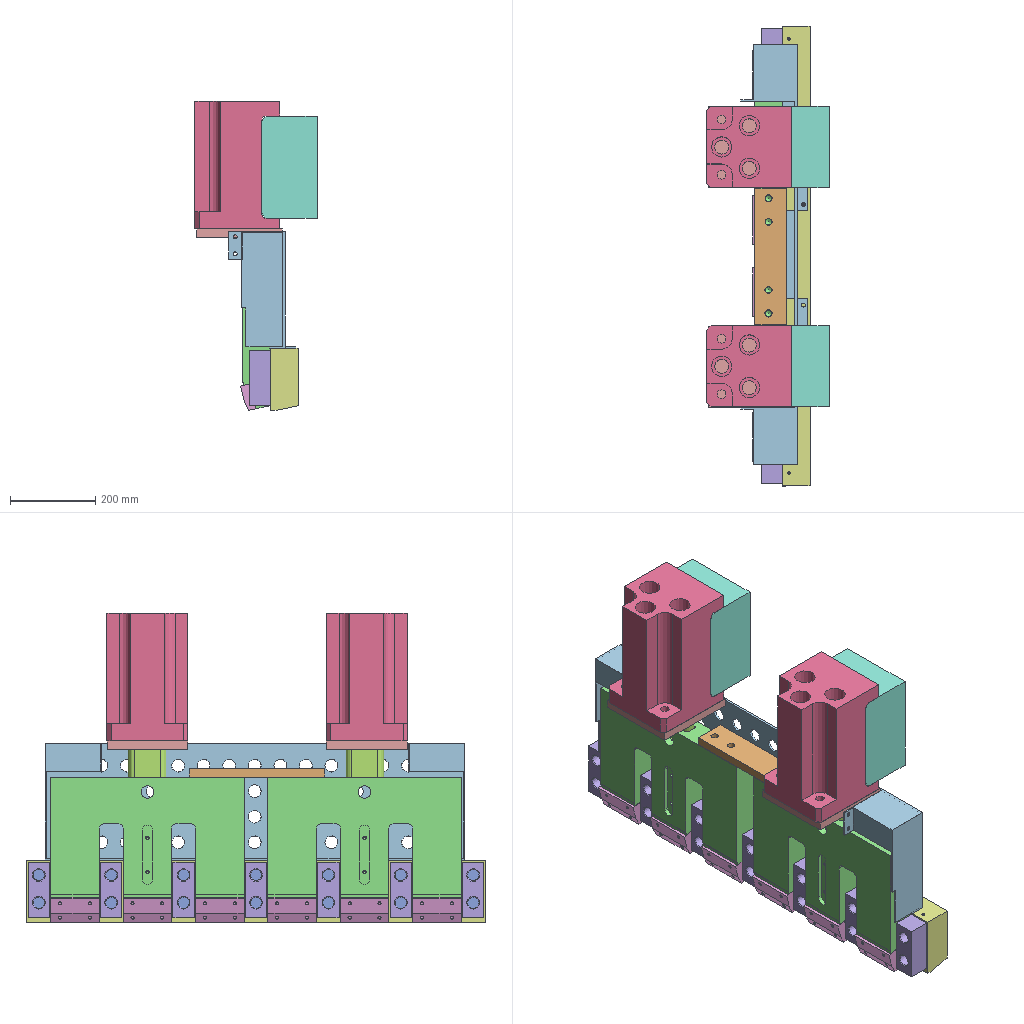Assembly | NX | 11 different items | 40 placed | box 288 x 1080 x 727 mm
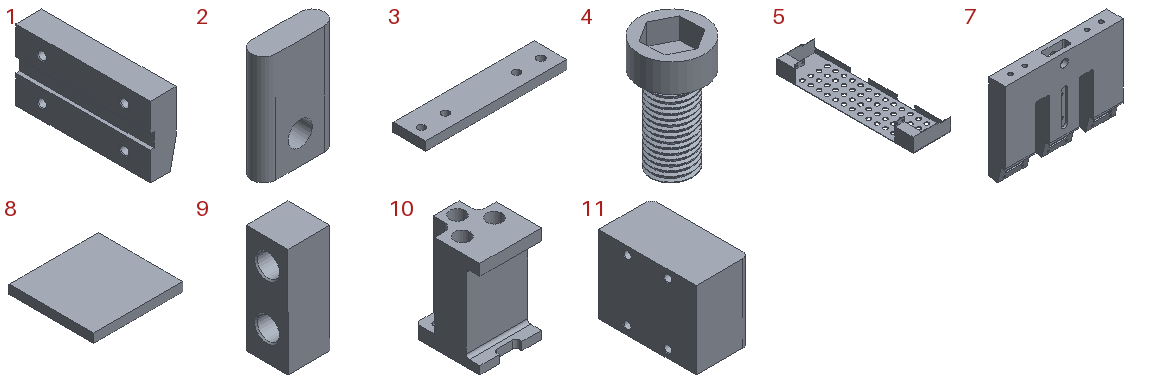Parts list (item | quantity | size | volume | features):
1 | x6 | 22 x 114 x 60 mm | 136204 mm3 | features SIMPLE HOLE 4, SYMBOLIC_THREAD 4, DATUM_CSYS 3, SKETCH 2, EXTRUDE 1, HOLE PACKAGE 1
2 | x2 | 90 x 30 x 135 mm | 317220 mm3 | features DATUM_CSYS 3, EXTRUDE 2, OFFSET_REGION 2, SKETCH 2, BLEND 1
3 | x1 | 319 x 74 x 20 mm | 453715 mm3 | features DATUM_CSYS 2, EXTRUDE 1, SKETCH 1
4 | x14 | 46 x 46 x 80 mm | 58631 mm3 | features DATUM_CSYS 4, EXTRUDE 3, SKETCH 3, THREADS 1
5 | x1 | 274 x 985 x 157 mm | 1535360 mm3 | features DATUM_CSYS 13, EXTRUDE 12, SKETCH 12, OFFSET_REGION 2
6 | x1 | - | - | features CBORE_HOLE 14, SIMPLE HOLE 6, SYMBOLIC_THREAD 6, DATUM_CSYS 4, SKETCH 3, HOLE PACKAGE 2, EXTRUDE 1
7 | x2 | 454 x 65 x 337.24 mm | 7495234 mm3 | features SIMPLE HOLE 20, SYMBOLIC_THREAD 20, DATUM_CSYS 11, SKETCH 10, EXTRUDE 6, HOLE PACKAGE 4, BLEND 1
8 | x2 | 200 x 190 x 20 mm | 760000 mm3 | features DATUM_CSYS 2, EXTRUDE 1, SKETCH 1
9 | x7 | 50 x 50 x 130 mm | 268964 mm3 | features DATUM_CSYS 3, SIMPLE HOLE 2, SKETCH 2, SYMBOLIC_THREAD 2, EXTRUDE 1, HOLE PACKAGE 1
10 | x2 | 190.5 x 200 x 300 mm | 6616630 mm3 | features DATUM_CSYS 6, SKETCH 5, EXTRUDE 4, CBORE_HOLE 3, BLEND 2, HOLE PACKAGE 2, SIMPLE HOLE 2, CHAMFER 1
11 | x2 | 130 x 240 x 190.5 mm | 5884853 mm3 | features SIMPLE HOLE 4, SYMBOLIC_THREAD 4, DATUM_CSYS 3, SKETCH 2, BLEND 1, EXTRUDE 1, HOLE PACKAGE 1
Mates (type | each side: item.copy, entity, surface, feature):
Touch | 7.1 face plane Extrude(1) | 6.1 face plane Extrude(1)